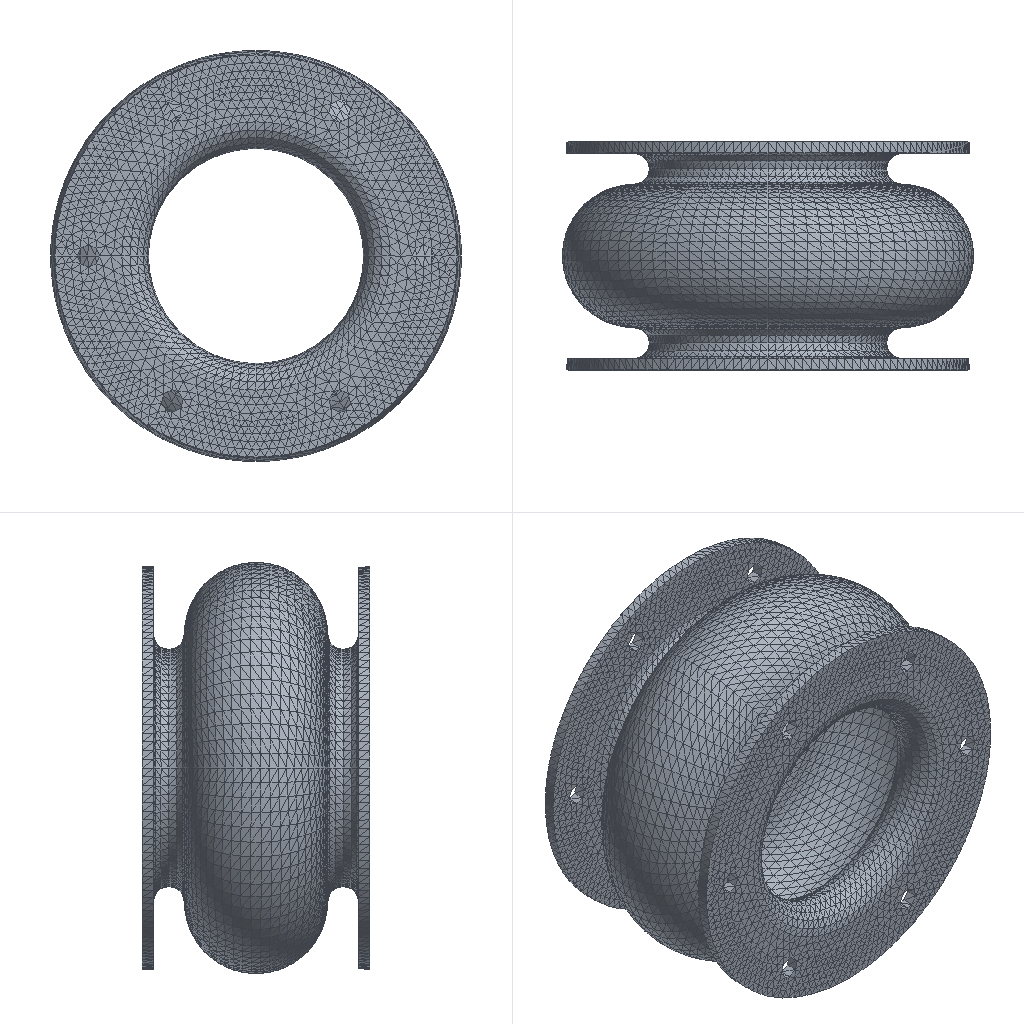Simulation study | abaqus
Set-up summary:
category,name,step,type,value,unit,region
solver,abaqus
solver,version,,,Abaqus/Explicit 2020
units,not stated in the deck,,not stated
analysis,deck,,transient,transient
load_step,Step-1,Step-1,transient
load_step,requested,,,1
mesh,nodes,,,24960
mesh,elements,,,67656
element_type,R3D3,,rigid,464
element_type,R3D4,,rigid,9515
element_type,C3D4H,,solid,57677
load,load commands in deck,,count,2
bc,support commands in deck,,count,7
material,CHAOTANXING,,in results
material,STEEL,,in results
check,setup vs results,,match,"per instance, exact: element labels, types and connectivity; labels of the nodes the elements use; coordinates of those nodes at SINGLE_PRECISION in 2 of 3 instance(s)"
Abaqus input file, long lists of numbers shortened:
*Heading
** Job name: Job-1 Model name: Model-1
** Generated by: Abaqus/CAE 2020
*Preprint, echo=NO, model=NO, history=NO, contact=NO
**
** PARTS
**
*Part, name=rigid-1
*Node
      1,           0.,          32.,         -60.
      2,           0.,          39.,         -53.
** (4025 more lines like these left out)
*Element, type=R3D4
 1,   1, 107, 709, 144
 2, 107,   2, 108, 709
** (3958 more lines like these left out)
*Element, type=R3D3
513,  887, 1006,  866
514, 1018,  945,  923
** (184 more lines like these left out)
*Node
   4028, -8.3668771e-15,          66.,           0.
*Nset, nset=rigid-1-RefPt_, internal
4028,
*Elset, elset=rigid-1, generate
    1,  4146,     1
*End Part
**
*Part, name=rigid-2
*Node
      1,  -51.961,         -46.,  -30.
      2,   -45.899,         -39.,  -26.5
** (5670 more lines like these left out)
*Element, type=R3D4
 1,   1, 143, 827, 176
 2, 143,   2, 144, 827
** (5553 more lines like these left out)
*Element, type=R3D3
497,    6,  919,  409
498,    5,  923,  209
** (276 more lines like these left out)
*Node
   5673, -0.00025,         -66., 0.000433
*Nset, nset=rigid-2-RefPt_, internal
5673,
*Elset, elset=rigid-2, generate
    1,  5833,     1
*End Part
**
*Part, name=work-1
*Node
      1,         -60.,          32.,           0.
      2,  -50.253,          32.,           0.
** (15257 more lines like these left out)
*Element, type=C3D4H
   1,  2811, 11199, 11200,  3128
   2,  3158, 11201, 11202,  3178
** (57675 more lines like these left out)
*Nset, nset=Set-7, generate
     1,  15259,      1
*Elset, elset=Set-7, generate
     1,  57677,      1
** Section: chaotanxing
*Solid Section, elset=Set-7, material=chaotanxing
,
*End Part
**
**
** ASSEMBLY
**
*Assembly, name=Assembly
**
*Instance, name=work-1-1, part=work-1
*End Instance
**
*Instance, name=rigid-2-1, part=rigid-2
*End Instance
**
*Instance, name=rigid-1-1, part=rigid-1
*End Instance
**
*Nset, nset=Set-1, instance=rigid-2-1
 5673,
*Nset, nset=Set-4, instance=rigid-1-1
 4028,
*Elset, elset=_Surf-12_S3, internal, instance=work-1-1
    20,    28,    59,    63,    78,    82,   116,   127,   177,   188,   189,   198,   211,   240,   266,   279
   333,   347,   361,   372,   414,   472,   500,   522,   592,   603,   607,   611,   627,   633,   647,   649
** (182 more lines like these left out)
*Elset, elset=_Surf-12_S4, internal, instance=work-1-1
   384,  1348,  1401,  1409,  1413,  1420,  1686,  1765,  1772,  1777,  1837,  1839,  1855,  1864,  1989,  2001
  2047,  2160,  2170,  2176,  2302,  2346,  2379,  2403,  2407,  2408,  2498,  2523,  2632,  2724,  2777,  2818
** (15 more lines like these left out)
*Elset, elset=_Surf-12_S2, internal, instance=work-1-1
   288,  1013,  1295,  1723,  1753,  1813,  1843,  1849,  1862,  2002,  2033,  2046,  2124,  2133,  2281,  2358
  2392,  2397,  2409,  2458,  2490,  2507,  2540,  2565,  2566,  2567,  2605,  2633,  2653,  2663,  2669,  2716
** (15 more lines like these left out)
*Elset, elset=_Surf-12_S1, internal, instance=work-1-1
    40,   166,   728,   748,   777,   838,   884,  1180,  1212,  1251,  1543,  1690,  1695,  1771,  1814,  1871
  1991,  2040,  2268,  2342,  2351,  2374,  2427,  2474,  2611,  2696,  2741,  2834,  2855,  2914,  3311,  3352
** (13 more lines like these left out)
*Surface, type=ELEMENT, name=Surf-12
_Surf-12_S3, S3
_Surf-12_S4, S4
_Surf-12_S2, S2
_Surf-12_S1, S1
*Elset, elset=_m_Surf-1_SPOS, internal, instance=rigid-2-1, generate
 1800,  5729,     1
*Surface, type=ELEMENT, name=m_Surf-1
_m_Surf-1_SPOS, SPOS
*Elset, elset=_m_Surf-3_SPOS, internal, instance=rigid-2-1, generate
 497,  739,    1
*Surface, type=ELEMENT, name=m_Surf-3
_m_Surf-3_SPOS, SPOS
*Elset, elset=_m_Surf-9_SPOS, internal, instance=rigid-2-1, generate
  740,  1044,     1
*Surface, type=ELEMENT, name=m_Surf-9
_m_Surf-9_SPOS, SPOS
*Elset, elset=_m_Surf-14_SPOS, internal, instance=rigid-1-1, generate
 513,  796,    1
*Surface, type=ELEMENT, name=m_Surf-14
_m_Surf-14_SPOS, SPOS
*Elset, elset=_m_Surf-15_SPOS, internal, instance=rigid-1-1, generate
  797,  1089,     1
*Surface, type=ELEMENT, name=m_Surf-15
_m_Surf-15_SPOS, SPOS
*Elset, elset=_m_Surf-16_SPOS, internal, instance=rigid-1-1, generate
 2349,  4081,     1
*Surface, type=ELEMENT, name=m_Surf-16
_m_Surf-16_SPOS, SPOS
*Elset, elset=_s_Surf-1_S3, internal, instance=work-1-1
  3908,  3917,  3926,  3936,  3937,  3951,  3995,  4005,  4042,  4053,  4059,  4069,  4075,  4110,  4113,  4123
  4150,  4187,  4190,  4216,  4225,  4230,  4237,  4245,  4274,  4277,  4351,  4365,  4389,  4421,  4424,  4453
** (114 more lines like these left out)
*Elset, elset=_s_Surf-1_S4, internal, instance=work-1-1
  3915,  4709,  4955,  5700,  5809, 10745, 10927, 11327, 11634, 12034, 12315, 12366, 28820, 29570, 30514, 30638
 30762, 30785, 32089, 32769, 32964, 32968, 33582, 33746, 33764, 37349, 37630, 37729, 38077, 38401, 38684, 38719
** (1 more lines like these left out)
*Elset, elset=_s_Surf-1_S1, internal, instance=work-1-1
  4984,  5301,  5323,  5921, 11050, 11936, 28681, 32732, 37312, 39032, 52777
*Elset, elset=_s_Surf-1_S2, internal, instance=work-1-1
  4995,  4999,  5783, 11559, 11586, 11593, 11835, 11845, 12026, 12033, 12072, 12126, 12201, 12253, 30012, 30731
 38832, 39028, 39489, 50390, 50786, 51330, 51876, 52567, 52619
*Surface, type=ELEMENT, name=s_Surf-1
_s_Surf-1_S3, S3
_s_Surf-1_S4, S4
_s_Surf-1_S2, S2
_s_Surf-1_S1, S1
*Elset, elset=_s_Surf-3_S1, internal, instance=work-1-1
  3927,  4546, 10238, 10270, 11281, 11583, 11808, 11840, 12334, 12393, 12397, 28386, 29501, 29698, 29860, 30102
 30450, 31291, 33818, 39483, 51635, 51640, 52121
*Elset, elset=_s_Surf-3_S3, internal, instance=work-1-1
  3932,  4040,  4147,  4178,  4210,  4212,  4307,  4309,  4350,  4387,  4425,  4442,  4577,  4630,  4631,  4644
  4645,  4684,  4734,  4740,  4794,  4828,  4859,  4891,  4899,  4901,  4905,  4912,  4913,  4929,  4982,  5022
** (114 more lines like these left out)
*Elset, elset=_s_Surf-3_S4, internal, instance=work-1-1
  4907,  5196,  5241,  5270,  5311,  5492,  5532,  5565,  5901,  5987,  6119, 10228, 10319, 10412, 10541, 10790
 10953, 11013, 11194, 11196, 11285, 11418, 12247, 12469, 12498, 12533, 28823, 28957, 29139, 29266, 29425, 29453
** (4 more lines like these left out)
*Elset, elset=_s_Surf-3_S2, internal, instance=work-1-1
  5416,  5721,  5729,  6150, 10173, 10476, 10618, 11153, 11321, 11394, 11430, 11884, 12514, 12580, 12643, 12673
 29043, 29134, 29205, 29639, 29940, 30093, 30331, 30784, 32617, 32624, 33452, 38023, 38451, 38569, 39142, 39332
** (1 more lines like these left out)
*Surface, type=ELEMENT, name=s_Surf-3
_s_Surf-3_S1, S1
_s_Surf-3_S3, S3
_s_Surf-3_S4, S4
_s_Surf-3_S2, S2
*Elset, elset=_s_Surf-5_S2, internal, instance=work-1-1
 12788, 15103, 17125, 17254, 17623, 17629, 17794, 17803, 18069, 22006, 22580, 22808, 23391, 23559, 24069, 36424
 36531, 37019, 45026, 45606, 45643, 45736, 45844, 46404, 46521, 46951, 47244, 48155, 48357, 48529, 48616, 48802
** (1 more lines like these left out)
*Elset, elset=_s_Surf-5_S3, internal, instance=work-1-1
 12845, 12869, 12895, 12910, 12916, 12969, 13005, 13059, 13081, 13092, 13102, 13104, 13106, 13182, 13240, 13243
 13255, 13256, 13267, 13273, 13297, 13310, 13312, 13332, 13367, 13369, 13370, 13394, 13400, 13428, 13434, 13437
** (117 more lines like these left out)
*Elset, elset=_s_Surf-5_S4, internal, instance=work-1-1
 13091, 13133, 13438, 13692, 14258, 14285, 14371, 14658, 14952, 15180, 16531, 16580, 16738, 17590, 22938, 23089
 23725, 24194, 24316, 24320, 24408, 34859, 34914, 34919, 34921, 34942, 34949, 35048, 35075, 35290, 35366, 35432
** (2 more lines like these left out)
*Elset, elset=_s_Surf-5_S1, internal, instance=work-1-1
 13783, 14114, 14235, 14446, 15108, 16288, 16453, 16686, 17583, 23098, 23886, 24152, 24588, 34736, 35961, 36044
 44466, 44550, 45999, 46525, 46680, 46926, 47214, 48117, 48148
*Surface, type=ELEMENT, name=s_Surf-5
_s_Surf-5_S2, S2
_s_Surf-5_S3, S3
_s_Surf-5_S4, S4
_s_Surf-5_S1, S1
*Elset, elset=_s_Surf-7_S3, internal, instance=work-1-1
 12893, 13054, 13088, 13181, 13242, 13380, 13403, 13449, 13591, 13593, 13680, 13780, 13784, 13870, 13876, 13878
 13901, 13903, 13951, 13993, 14053, 14060, 14066, 14070, 14075, 14092, 14104, 14108, 14125, 14129, 14132, 14142
** (114 more lines like these left out)
*Elset, elset=_s_Surf-7_S4, internal, instance=work-1-1
 13117, 13540, 13594, 13598, 13937, 14491, 14886, 14958, 15133, 15177, 16017, 16613, 16774, 16963, 17364, 17763
 17796, 21864, 22137, 22740, 22759, 23215, 23218, 24092, 24317, 24322, 34428, 35143, 35563, 35993, 36194, 36840
** (1 more lines like these left out)
*Elset, elset=_s_Surf-7_S2, internal, instance=work-1-1
 14915, 15102, 15562, 15603, 16657, 16818, 16821, 16833, 16943, 16972, 17046, 18152, 21880, 23753, 24142, 35202
 35455, 36024, 36403, 36635, 36844, 46373, 46981, 49321, 49678, 49921, 49924
*Elset, elset=_s_Surf-7_S1, internal, instance=work-1-1
 13070, 14001, 14788, 16868, 16944, 16950, 18025, 18165, 21875, 23925, 46382, 48101, 48467, 49599
*Surface, type=ELEMENT, name=s_Surf-7
_s_Surf-7_S3, S3
_s_Surf-7_S4, S4
_s_Surf-7_S2, S2
_s_Surf-7_S1, S1
*Elset, elset=_s_Surf-9_S3, internal, instance=work-1-1
     9,    58,    95,   112,   156,   218,   233,   238,   323,   378,   412,   435,   447,   448,   450,   451
   509,   523,   533,   537,   557,   582,   585,   600,   604,   637,   704,   731,   735,   736,   742,   762
** (229 more lines like these left out)
*Elset, elset=_s_Surf-9_S1, internal, instance=work-1-1
    34,   204,   210,   468,   727,  1090,  1105,  1243,  1320,  1384,  1419,  1660,  1702,  1868,  1880,  1969
  2007,  2324,  2434,  2505,  2517,  2912,  3067,  3194,  3313,  3347,  3363,  3581,  3623,  3775,  6537,  6595
** (10 more lines like these left out)
*Elset, elset=_s_Surf-9_S4, internal, instance=work-1-1
    56,   103,   111,   114,   322,   369,   393,   642,   671,   746,   774,   796,   830,   972,  1094,  1106
  1107,  1381,  1403,  1507,  1508,  1578,  1664,  1683,  1790,  1819,  1948,  2027,  2135,  2489,  2532,  2544
** (20 more lines like these left out)
*Elset, elset=_s_Surf-9_S2, internal, instance=work-1-1
   185,   190,   459,   546,   672,  1368,  1509,  1728,  1737,  1762,  1879,  2287,  2337,  2368,  2415,  2534
  2616,  2617,  2628,  2655,  2662,  2667,  2688,  2715,  2740,  2879,  2980,  3030,  3223,  3480,  3650,  6637
** (10 more lines like these left out)
*Surface, type=ELEMENT, name=s_Surf-9
_s_Surf-9_S3, S3
_s_Surf-9_S1, S1
_s_Surf-9_S4, S4
_s_Surf-9_S2, S2
*Rigid Body, ref node=rigid-2-1.rigid-2-RefPt_, elset=rigid-2-1.rigid-2
*Rigid Body, ref node=rigid-1-1.rigid-1-RefPt_, elset=rigid-1-1.rigid-1
** Constraint: Constraint-1
*Tie, name=Constraint-1, adjust=yes
s_Surf-1, m_Surf-1
** Constraint: Constraint-2
*Tie, name=Constraint-2, adjust=yes
s_Surf-3, m_Surf-3
** Constraint: Constraint-3
*Tie, name=Constraint-3, adjust=yes
s_Surf-5, m_Surf-15
** Constraint: Constraint-4
*Tie, name=Constraint-4, adjust=yes
s_Surf-7, m_Surf-16
*End Assembly
*Amplitude, name=Amp-1, definition=PERIODIC
1,            62.8,              0.,              0.
           157.,              0.
*Amplitude, name=Amp-2
             0.,              0.,            0.05,              1.
**
** MATERIALS
**
*Material, name=chaotanxing
*Density
 2e-09,
*Hyperelastic, mooney-rivlin
 0.805, 0.194,    0.
*Material, name=steel
*Density
 7.8e-09,
*Elastic
210000., 0.3
**
** INTERACTION PROPERTIES
**
*Surface Interaction, name=IntProp-1
*Friction
 0.4,
*Surface Behavior, pressure-overclosure=HARD
** ----------------------------------------------------------------
**
** STEP: Step-1
**
*Step, name=Step-1, nlgeom=YES
*Dynamic, Explicit
, 0.05
*Bulk Viscosity
0.06, 1.2
**
** BOUNDARY CONDITIONS
**
** Name: BC-1 Type: 对称/反对称/完全固定
*Boundary
Set-1, ENCASTRE
** Name: BC-2 Type: 速度/角速度
*Boundary, amplitude=Amp-1, type=VELOCITY
Set-4, 1, 1
Set-4, 2, 2, 1.
Set-4, 3, 3
Set-4, 4, 4
Set-4, 5, 5
Set-4, 6, 6
**
** LOADS
**
** Name: Load-1   Type: Pressure
*Dsload, amplitude=Amp-2
Surf-12, P, 0.1
**
** INTERACTIONS
**
** Interaction: Int-1
*Contact Pair, interaction=IntProp-1, mechanical constraint=PENALTY, cpset=Int-1
m_Surf-9, s_Surf-9
** Interaction: Int-2
*Contact Pair, interaction=IntProp-1, mechanical constraint=PENALTY, cpset=Int-2
m_Surf-14, s_Surf-9
**
** OUTPUT REQUESTS
**
*Restart, write, number interval=1, time marks=NO
**
** FIELD OUTPUT: F-Output-1
**
*Output, field, number interval=50
*Node Output
A, RF, RM, RT, U, V
*Element Output, directions=YES
E, EVF, LE, MISES, PE, PEEQ, PEEQVAVG, PEVAVG, S, SVAVG
*Contact Output
CDISP, CSTRESS
**
** HISTORY OUTPUT: H-Output-1
**
*Output, history, variable=PRESELECT, frequency=10
*End Step
Results summary:
result,step,Step-1,completed,increments=57727 time=0.05/0.05
result,analysis,,,transient
result,last_loadstep,,,1
result,primary field,,,U
result,reaction total,,FX,1.332,model units
result,reaction total,,FY,-25.797,model units
result,reaction total,,FZ,-1.56,model units